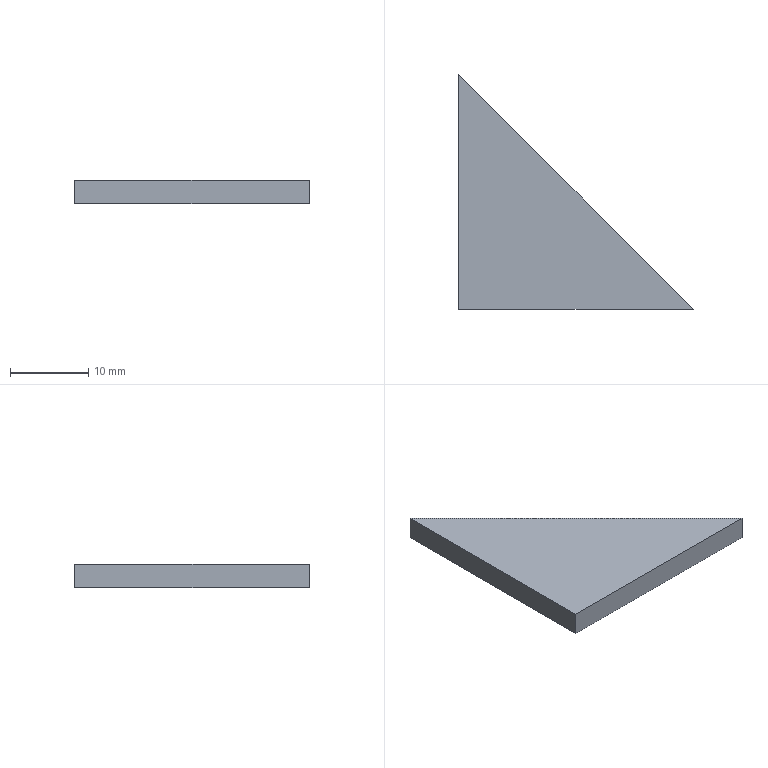Part | STEP file | 7471206 | 1 solid | 5 faces | box 30 x 30 x 3 mm | volume 1350 mm3 | plane 5
STEP:
#1=CARTESIAN_POINT('',(0.,0.,0.));
#2=DIRECTION('',(0.,0.,1.));
#3=DIRECTION('',(1.,0.,0.));
#4=AXIS2_PLACEMENT_3D('',#1,#2,#3);
#5=CARTESIAN_POINT('',(7.374,-18.331,0.));
#6=VERTEX_POINT('',#5);
#7=CARTESIAN_POINT('',(-22.626,11.669,0.));
#8=VERTEX_POINT('',#7);
#9=CARTESIAN_POINT('',(7.374,-18.331,0.));
#10=DIRECTION('',(-0.7071,0.7071,0.));
#11=VECTOR('',#10,1.);
#12=LINE('',#9,#11);
#13=CARTESIAN_POINT('',(7.374,-18.331,3.));
#14=DIRECTION('',(-0.7071,-0.7071,0.));
#15=DIRECTION('',(0.7071,-0.7071,0.));
#16=AXIS2_PLACEMENT_3D('',#13,#14,#15);
#17=PLANE('',#16);
#18=CARTESIAN_POINT('',(0.,-3.));
#19=DIRECTION('',(-1.,0.));
#20=VECTOR('',#19,1.);
#21=LINE('',#18,#20);
#22=(GEOMETRIC_REPRESENTATION_CONTEXT(2)PARAMETRIC_REPRESENTATION_CONTEXT()REPRESENTATION_CONTEXT('',''));
#23=DEFINITIONAL_REPRESENTATION('',(#21),#22);
#24=PCURVE('',#17,#23);
#25=CARTESIAN_POINT('',(0.,0.,0.));
#26=DIRECTION('',(0.,0.,1.));
#27=DIRECTION('',(1.,0.,0.));
#28=AXIS2_PLACEMENT_3D('',#25,#26,#27);
#29=PLANE('',#28);
#30=CARTESIAN_POINT('',(7.374,-18.331));
#31=DIRECTION('',(-0.7071,0.7071));
#32=VECTOR('',#31,1.);
#33=LINE('',#30,#32);
#34=(GEOMETRIC_REPRESENTATION_CONTEXT(2)PARAMETRIC_REPRESENTATION_CONTEXT()REPRESENTATION_CONTEXT('',''));
#35=DEFINITIONAL_REPRESENTATION('',(#33),#34);
#36=PCURVE('',#29,#35);
#37=SURFACE_CURVE('',#12,(#24,#36),.PCURVE_S1.);
#38=EDGE_CURVE('',#6,#8,#37,.T.);
#39=ORIENTED_EDGE('',*,*,#38,.T.);
#40=CARTESIAN_POINT('',(-22.626,11.669,3.));
#41=VERTEX_POINT('',#40);
#42=CARTESIAN_POINT('',(-22.626,11.669,3.));
#43=DIRECTION('',(0.,0.,-1.));
#44=VECTOR('',#43,1.);
#45=LINE('',#42,#44);
#46=CARTESIAN_POINT('',(-42.426,0.));
#47=DIRECTION('',(0.,-1.));
#48=VECTOR('',#47,1.);
#49=LINE('',#46,#48);
#50=(GEOMETRIC_REPRESENTATION_CONTEXT(2)PARAMETRIC_REPRESENTATION_CONTEXT()REPRESENTATION_CONTEXT('',''));
#51=DEFINITIONAL_REPRESENTATION('',(#49),#50);
#52=PCURVE('',#17,#51);
#53=CARTESIAN_POINT('',(-22.626,11.669,3.));
#54=DIRECTION('',(1.,0.,0.));
#55=DIRECTION('',(0.,1.,0.));
#56=AXIS2_PLACEMENT_3D('',#53,#54,#55);
#57=PLANE('',#56);
#58=CARTESIAN_POINT('',(0.,0.));
#59=DIRECTION('',(0.,-1.));
#60=VECTOR('',#59,1.);
#61=LINE('',#58,#60);
#62=(GEOMETRIC_REPRESENTATION_CONTEXT(2)PARAMETRIC_REPRESENTATION_CONTEXT()REPRESENTATION_CONTEXT('',''));
#63=DEFINITIONAL_REPRESENTATION('',(#61),#62);
#64=PCURVE('',#57,#63);
#65=SURFACE_CURVE('',#45,(#52,#64),.PCURVE_S1.);
#66=EDGE_CURVE('',#41,#8,#65,.T.);
#67=ORIENTED_EDGE('',*,*,#66,.F.);
#68=CARTESIAN_POINT('',(7.374,-18.331,3.));
#69=VERTEX_POINT('',#68);
#70=CARTESIAN_POINT('',(7.374,-18.331,3.));
#71=DIRECTION('',(-0.7071,0.7071,0.));
#72=VECTOR('',#71,1.);
#73=LINE('',#70,#72);
#74=CARTESIAN_POINT('',(0.,0.));
#75=DIRECTION('',(-1.,0.));
#76=VECTOR('',#75,1.);
#77=LINE('',#74,#76);
#78=(GEOMETRIC_REPRESENTATION_CONTEXT(2)PARAMETRIC_REPRESENTATION_CONTEXT()REPRESENTATION_CONTEXT('',''));
#79=DEFINITIONAL_REPRESENTATION('',(#77),#78);
#80=PCURVE('',#17,#79);
#81=CARTESIAN_POINT('',(0.,0.,3.));
#82=DIRECTION('',(0.,0.,1.));
#83=DIRECTION('',(1.,0.,0.));
#84=AXIS2_PLACEMENT_3D('',#81,#82,#83);
#85=PLANE('',#84);
#86=CARTESIAN_POINT('',(7.374,-18.331));
#87=DIRECTION('',(-0.7071,0.7071));
#88=VECTOR('',#87,1.);
#89=LINE('',#86,#88);
#90=(GEOMETRIC_REPRESENTATION_CONTEXT(2)PARAMETRIC_REPRESENTATION_CONTEXT()REPRESENTATION_CONTEXT('',''));
#91=DEFINITIONAL_REPRESENTATION('',(#89),#90);
#92=PCURVE('',#85,#91);
#93=SURFACE_CURVE('',#73,(#80,#92),.PCURVE_S1.);
#94=EDGE_CURVE('',#69,#41,#93,.T.);
#95=ORIENTED_EDGE('',*,*,#94,.F.);
#96=CARTESIAN_POINT('',(7.374,-18.331,3.));
#97=DIRECTION('',(0.,0.,-1.));
#98=VECTOR('',#97,1.);
#99=LINE('',#96,#98);
#100=CARTESIAN_POINT('',(0.,0.));
#101=DIRECTION('',(0.,-1.));
#102=VECTOR('',#101,1.);
#103=LINE('',#100,#102);
#104=(GEOMETRIC_REPRESENTATION_CONTEXT(2)PARAMETRIC_REPRESENTATION_CONTEXT()REPRESENTATION_CONTEXT('',''));
#105=DEFINITIONAL_REPRESENTATION('',(#103),#104);
#106=PCURVE('',#17,#105);
#107=CARTESIAN_POINT('',(-22.626,-18.331,3.));
#108=DIRECTION('',(0.,1.,0.));
#109=DIRECTION('',(0.,0.,1.));
#110=AXIS2_PLACEMENT_3D('',#107,#108,#109);
#111=PLANE('',#110);
#112=CARTESIAN_POINT('',(0.,30.));
#113=DIRECTION('',(-1.,0.));
#114=VECTOR('',#113,1.);
#115=LINE('',#112,#114);
#116=(GEOMETRIC_REPRESENTATION_CONTEXT(2)PARAMETRIC_REPRESENTATION_CONTEXT()REPRESENTATION_CONTEXT('',''));
#117=DEFINITIONAL_REPRESENTATION('',(#115),#116);
#118=PCURVE('',#111,#117);
#119=SURFACE_CURVE('',#99,(#106,#118),.PCURVE_S1.);
#120=EDGE_CURVE('',#69,#6,#119,.T.);
#121=ORIENTED_EDGE('',*,*,#120,.T.);
#122=EDGE_LOOP('',(#39,#67,#95,#121));
#123=FACE_BOUND('',#122,.T.);
#124=ADVANCED_FACE('',(#123),#17,.F.);
#125=CARTESIAN_POINT('',(-22.626,-18.331,0.));
#126=VERTEX_POINT('',#125);
#127=CARTESIAN_POINT('',(-22.626,11.669,0.));
#128=DIRECTION('',(0.,-1.,0.));
#129=VECTOR('',#128,1.);
#130=LINE('',#127,#129);
#131=CARTESIAN_POINT('',(0.,-3.));
#132=DIRECTION('',(-1.,0.));
#133=VECTOR('',#132,1.);
#134=LINE('',#131,#133);
#135=(GEOMETRIC_REPRESENTATION_CONTEXT(2)PARAMETRIC_REPRESENTATION_CONTEXT()REPRESENTATION_CONTEXT('',''));
#136=DEFINITIONAL_REPRESENTATION('',(#134),#135);
#137=PCURVE('',#57,#136);
#138=CARTESIAN_POINT('',(-22.626,11.669));
#139=DIRECTION('',(0.,-1.));
#140=VECTOR('',#139,1.);
#141=LINE('',#138,#140);
#142=(GEOMETRIC_REPRESENTATION_CONTEXT(2)PARAMETRIC_REPRESENTATION_CONTEXT()REPRESENTATION_CONTEXT('',''));
#143=DEFINITIONAL_REPRESENTATION('',(#141),#142);
#144=PCURVE('',#29,#143);
#145=SURFACE_CURVE('',#130,(#137,#144),.PCURVE_S1.);
#146=EDGE_CURVE('',#8,#126,#145,.T.);
#147=ORIENTED_EDGE('',*,*,#146,.T.);
#148=CARTESIAN_POINT('',(-22.626,-18.331,3.));
#149=VERTEX_POINT('',#148);
#150=CARTESIAN_POINT('',(-22.626,-18.331,3.));
#151=DIRECTION('',(0.,0.,-1.));
#152=VECTOR('',#151,1.);
#153=LINE('',#150,#152);
#154=CARTESIAN_POINT('',(-30.,0.));
#155=DIRECTION('',(0.,-1.));
#156=VECTOR('',#155,1.);
#157=LINE('',#154,#156);
#158=(GEOMETRIC_REPRESENTATION_CONTEXT(2)PARAMETRIC_REPRESENTATION_CONTEXT()REPRESENTATION_CONTEXT('',''));
#159=DEFINITIONAL_REPRESENTATION('',(#157),#158);
#160=PCURVE('',#57,#159);
#161=CARTESIAN_POINT('',(0.,0.));
#162=DIRECTION('',(-1.,0.));
#163=VECTOR('',#162,1.);
#164=LINE('',#161,#163);
#165=(GEOMETRIC_REPRESENTATION_CONTEXT(2)PARAMETRIC_REPRESENTATION_CONTEXT()REPRESENTATION_CONTEXT('',''));
#166=DEFINITIONAL_REPRESENTATION('',(#164),#165);
#167=PCURVE('',#111,#166);
#168=SURFACE_CURVE('',#153,(#160,#167),.PCURVE_S1.);
#169=EDGE_CURVE('',#149,#126,#168,.T.);
#170=ORIENTED_EDGE('',*,*,#169,.F.);
#171=CARTESIAN_POINT('',(-22.626,11.669,3.));
#172=DIRECTION('',(0.,-1.,0.));
#173=VECTOR('',#172,1.);
#174=LINE('',#171,#173);
#175=CARTESIAN_POINT('',(0.,0.));
#176=DIRECTION('',(-1.,0.));
#177=VECTOR('',#176,1.);
#178=LINE('',#175,#177);
#179=(GEOMETRIC_REPRESENTATION_CONTEXT(2)PARAMETRIC_REPRESENTATION_CONTEXT()REPRESENTATION_CONTEXT('',''));
#180=DEFINITIONAL_REPRESENTATION('',(#178),#179);
#181=PCURVE('',#57,#180);
#182=CARTESIAN_POINT('',(-22.626,11.669));
#183=DIRECTION('',(0.,-1.));
#184=VECTOR('',#183,1.);
#185=LINE('',#182,#184);
#186=(GEOMETRIC_REPRESENTATION_CONTEXT(2)PARAMETRIC_REPRESENTATION_CONTEXT()REPRESENTATION_CONTEXT('',''));
#187=DEFINITIONAL_REPRESENTATION('',(#185),#186);
#188=PCURVE('',#85,#187);
#189=SURFACE_CURVE('',#174,(#181,#188),.PCURVE_S1.);
#190=EDGE_CURVE('',#41,#149,#189,.T.);
#191=ORIENTED_EDGE('',*,*,#190,.F.);
#192=ORIENTED_EDGE('',*,*,#66,.T.);
#193=EDGE_LOOP('',(#147,#170,#191,#192));
#194=FACE_BOUND('',#193,.T.);
#195=ADVANCED_FACE('',(#194),#57,.F.);
#196=CARTESIAN_POINT('',(-22.626,-18.331,0.));
#197=DIRECTION('',(1.,0.,0.));
#198=VECTOR('',#197,1.);
#199=LINE('',#196,#198);
#200=CARTESIAN_POINT('',(-3.,0.));
#201=DIRECTION('',(0.,1.));
#202=VECTOR('',#201,1.);
#203=LINE('',#200,#202);
#204=(GEOMETRIC_REPRESENTATION_CONTEXT(2)PARAMETRIC_REPRESENTATION_CONTEXT()REPRESENTATION_CONTEXT('',''));
#205=DEFINITIONAL_REPRESENTATION('',(#203),#204);
#206=PCURVE('',#111,#205);
#207=CARTESIAN_POINT('',(-22.626,-18.331));
#208=DIRECTION('',(1.,0.));
#209=VECTOR('',#208,1.);
#210=LINE('',#207,#209);
#211=(GEOMETRIC_REPRESENTATION_CONTEXT(2)PARAMETRIC_REPRESENTATION_CONTEXT()REPRESENTATION_CONTEXT('',''));
#212=DEFINITIONAL_REPRESENTATION('',(#210),#211);
#213=PCURVE('',#29,#212);
#214=SURFACE_CURVE('',#199,(#206,#213),.PCURVE_S1.);
#215=EDGE_CURVE('',#126,#6,#214,.T.);
#216=ORIENTED_EDGE('',*,*,#215,.T.);
#217=ORIENTED_EDGE('',*,*,#120,.F.);
#218=CARTESIAN_POINT('',(-22.626,-18.331,3.));
#219=DIRECTION('',(1.,0.,0.));
#220=VECTOR('',#219,1.);
#221=LINE('',#218,#220);
#222=CARTESIAN_POINT('',(0.,0.));
#223=DIRECTION('',(0.,1.));
#224=VECTOR('',#223,1.);
#225=LINE('',#222,#224);
#226=(GEOMETRIC_REPRESENTATION_CONTEXT(2)PARAMETRIC_REPRESENTATION_CONTEXT()REPRESENTATION_CONTEXT('',''));
#227=DEFINITIONAL_REPRESENTATION('',(#225),#226);
#228=PCURVE('',#111,#227);
#229=CARTESIAN_POINT('',(-22.626,-18.331));
#230=DIRECTION('',(1.,0.));
#231=VECTOR('',#230,1.);
#232=LINE('',#229,#231);
#233=(GEOMETRIC_REPRESENTATION_CONTEXT(2)PARAMETRIC_REPRESENTATION_CONTEXT()REPRESENTATION_CONTEXT('',''));
#234=DEFINITIONAL_REPRESENTATION('',(#232),#233);
#235=PCURVE('',#85,#234);
#236=SURFACE_CURVE('',#221,(#228,#235),.PCURVE_S1.);
#237=EDGE_CURVE('',#149,#69,#236,.T.);
#238=ORIENTED_EDGE('',*,*,#237,.F.);
#239=ORIENTED_EDGE('',*,*,#169,.T.);
#240=EDGE_LOOP('',(#216,#217,#238,#239));
#241=FACE_BOUND('',#240,.T.);
#242=ADVANCED_FACE('',(#241),#111,.F.);
#243=ORIENTED_EDGE('',*,*,#94,.T.);
#244=ORIENTED_EDGE('',*,*,#190,.T.);
#245=ORIENTED_EDGE('',*,*,#237,.T.);
#246=EDGE_LOOP('',(#243,#244,#245));
#247=FACE_BOUND('',#246,.T.);
#248=ADVANCED_FACE('',(#247),#85,.T.);
#249=ORIENTED_EDGE('',*,*,#38,.F.);
#250=ORIENTED_EDGE('',*,*,#215,.F.);
#251=ORIENTED_EDGE('',*,*,#146,.F.);
#252=EDGE_LOOP('',(#249,#250,#251));
#253=FACE_BOUND('',#252,.T.);
#254=ADVANCED_FACE('',(#253),#29,.F.);
#255=CLOSED_SHELL('',(#124,#195,#242,#248,#254));
#256=MANIFOLD_SOLID_BREP('',#255);
#257=(LENGTH_UNIT()NAMED_UNIT(*)SI_UNIT(.MILLI.,.METRE.));
#258=UNCERTAINTY_MEASURE_WITH_UNIT(LENGTH_MEASURE(0.0000001),#257,'','');
#259=(NAMED_UNIT(*)PLANE_ANGLE_UNIT()SI_UNIT($,.RADIAN.));
#260=(NAMED_UNIT(*)SI_UNIT($,.STERADIAN.)SOLID_ANGLE_UNIT());
#261=(GEOMETRIC_REPRESENTATION_CONTEXT(3)GLOBAL_UNCERTAINTY_ASSIGNED_CONTEXT((#258))GLOBAL_UNIT_ASSIGNED_CONTEXT((#257,#259,#260))REPRESENTATION_CONTEXT('',''));
#262=ADVANCED_BREP_SHAPE_REPRESENTATION('',(#4,#256),#261);